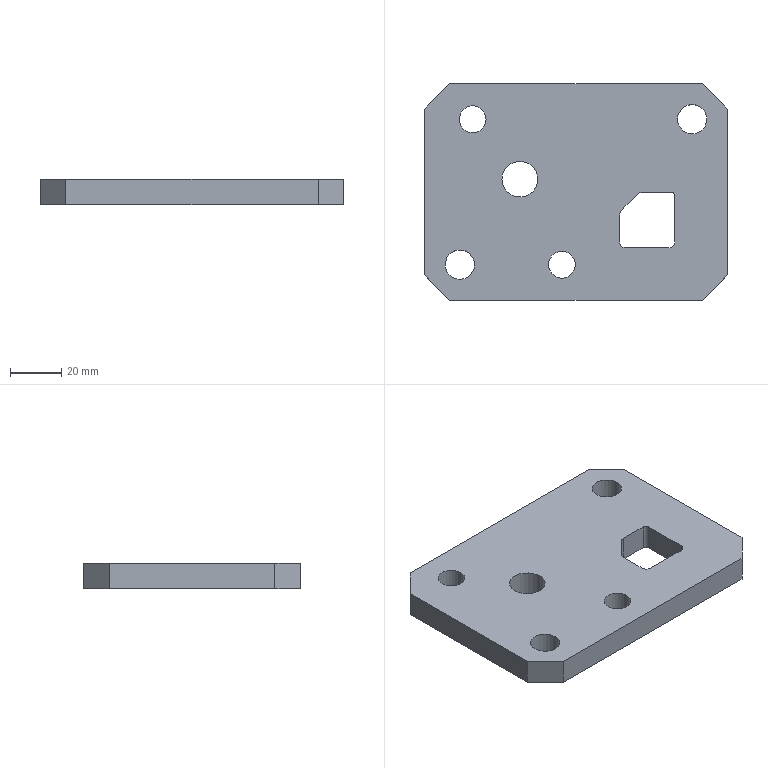Part | NX | features 23 2 | 1 solid | 25 faces | box 119 x 85 x 10 mm | volume 89428 mm3 | plane 15 | cylinder 10 | commonest cylinder face diameters 4.6 x2 5.6 x2 10.5 x2 11.509 x2 3 x1 14 x1
STEP:
#1=CARTESIAN_POINT('',(80.029,-411.95,-33.5));
#2=VERTEX_POINT('',#1);
#3=CARTESIAN_POINT('',(87.029,-411.95,-33.5));
#4=DIRECTION('',(0.,0.,-1.));
#5=DIRECTION('',(-1.,0.,0.));
#6=AXIS2_PLACEMENT_3D('',#3,#4,#5);
#7=CIRCLE('',#6,7.);
#8=EDGE_CURVE('',#2,#2,#7,.T.);
#9=ORIENTED_EDGE('',*,*,#8,.F.);
#10=EDGE_LOOP('',(#9));
#11=FACE_BOUND('',#10,.T.);
#12=CARTESIAN_POINT('',(80.029,-411.95,-43.5));
#13=VERTEX_POINT('',#12);
#14=CARTESIAN_POINT('',(87.029,-411.95,-43.5));
#15=DIRECTION('',(0.,0.,-1.));
#16=DIRECTION('',(-1.,0.,0.));
#17=AXIS2_PLACEMENT_3D('',#14,#15,#16);
#18=CIRCLE('',#17,7.);
#19=EDGE_CURVE('',#13,#13,#18,.T.);
#20=ORIENTED_EDGE('',*,*,#19,.T.);
#21=EDGE_LOOP('',(#20));
#22=FACE_BOUND('',#21,.T.);
#23=CARTESIAN_POINT('',(87.029,-411.95,-33.5));
#24=DIRECTION('',(0.,0.,1.));
#25=DIRECTION('',(1.,0.,0.));
#26=AXIS2_PLACEMENT_3D('',#23,#24,#25);
#27=CYLINDRICAL_SURFACE('',#26,7.);
#28=ADVANCED_FACE('',(#11,#22),#27,.F.);
#29=CARTESIAN_POINT('',(49.529,-449.45,-33.5));
#30=VERTEX_POINT('',#29);
#31=CARTESIAN_POINT('',(49.529,-384.45,-33.5));
#32=VERTEX_POINT('',#31);
#33=CARTESIAN_POINT('',(49.529,-411.95,-33.5));
#34=DIRECTION('',(0.,1.,0.));
#35=VECTOR('',#34,1000.);
#36=LINE('',#33,#35);
#37=EDGE_CURVE('',#30,#32,#36,.T.);
#38=ORIENTED_EDGE('',*,*,#37,.T.);
#39=CARTESIAN_POINT('',(49.529,-384.45,-43.5));
#40=VERTEX_POINT('',#39);
#41=CARTESIAN_POINT('',(49.529,-384.45,-33.5));
#42=DIRECTION('',(0.,0.,1.));
#43=VECTOR('',#42,1000.);
#44=LINE('',#41,#43);
#45=EDGE_CURVE('',#40,#32,#44,.T.);
#46=ORIENTED_EDGE('',*,*,#45,.F.);
#47=CARTESIAN_POINT('',(49.529,-449.45,-43.5));
#48=VERTEX_POINT('',#47);
#49=CARTESIAN_POINT('',(49.529,-377.506,-43.5));
#50=DIRECTION('',(0.,1.,0.));
#51=VECTOR('',#50,1000.);
#52=LINE('',#49,#51);
#53=EDGE_CURVE('',#48,#40,#52,.T.);
#54=ORIENTED_EDGE('',*,*,#53,.F.);
#55=CARTESIAN_POINT('',(49.529,-449.45,-33.5));
#56=DIRECTION('',(0.,0.,-1.));
#57=VECTOR('',#56,1000.);
#58=LINE('',#55,#57);
#59=EDGE_CURVE('',#30,#48,#58,.T.);
#60=ORIENTED_EDGE('',*,*,#59,.F.);
#61=EDGE_LOOP('',(#38,#46,#54,#60));
#62=FACE_BOUND('',#61,.T.);
#63=CARTESIAN_POINT('',(49.529,-411.95,-33.5));
#64=DIRECTION('',(1.,0.,0.));
#65=DIRECTION('',(0.,1.,0.));
#66=AXIS2_PLACEMENT_3D('',#63,#64,#65);
#67=PLANE('',#66);
#68=ADVANCED_FACE('',(#62),#67,.F.);
#69=CARTESIAN_POINT('',(158.529,-459.45,-33.5));
#70=VERTEX_POINT('',#69);
#71=CARTESIAN_POINT('',(59.529,-459.45,-33.5));
#72=VERTEX_POINT('',#71);
#73=CARTESIAN_POINT('',(87.029,-459.45,-33.5));
#74=DIRECTION('',(-1.,0.,0.));
#75=VECTOR('',#74,1000.);
#76=LINE('',#73,#75);
#77=EDGE_CURVE('',#70,#72,#76,.T.);
#78=ORIENTED_EDGE('',*,*,#77,.T.);
#79=CARTESIAN_POINT('',(59.529,-459.45,-43.5));
#80=VERTEX_POINT('',#79);
#81=CARTESIAN_POINT('',(59.529,-459.45,-33.5));
#82=DIRECTION('',(0.,0.,1.));
#83=VECTOR('',#82,1000.);
#84=LINE('',#81,#83);
#85=EDGE_CURVE('',#80,#72,#84,.T.);
#86=ORIENTED_EDGE('',*,*,#85,.F.);
#87=CARTESIAN_POINT('',(158.529,-459.45,-43.5));
#88=VERTEX_POINT('',#87);
#89=CARTESIAN_POINT('',(119.455,-459.45,-43.5));
#90=DIRECTION('',(-1.,0.,0.));
#91=VECTOR('',#90,1000.);
#92=LINE('',#89,#91);
#93=EDGE_CURVE('',#88,#80,#92,.T.);
#94=ORIENTED_EDGE('',*,*,#93,.F.);
#95=CARTESIAN_POINT('',(158.529,-459.45,-33.5));
#96=DIRECTION('',(0.,0.,-1.));
#97=VECTOR('',#96,1000.);
#98=LINE('',#95,#97);
#99=EDGE_CURVE('',#70,#88,#98,.T.);
#100=ORIENTED_EDGE('',*,*,#99,.F.);
#101=EDGE_LOOP('',(#78,#86,#94,#100));
#102=FACE_BOUND('',#101,.T.);
#103=CARTESIAN_POINT('',(87.029,-459.45,-33.5));
#104=DIRECTION('',(0.,1.,0.));
#105=DIRECTION('',(-1.,0.,0.));
#106=AXIS2_PLACEMENT_3D('',#103,#104,#105);
#107=PLANE('',#106);
#108=ADVANCED_FACE('',(#102),#107,.F.);
#109=CARTESIAN_POINT('',(168.529,-384.45,-33.5));
#110=VERTEX_POINT('',#109);
#111=CARTESIAN_POINT('',(168.529,-449.45,-33.5));
#112=VERTEX_POINT('',#111);
#113=CARTESIAN_POINT('',(168.529,-411.95,-33.5));
#114=DIRECTION('',(0.,-1.,0.));
#115=VECTOR('',#114,1000.);
#116=LINE('',#113,#115);
#117=EDGE_CURVE('',#110,#112,#116,.T.);
#118=ORIENTED_EDGE('',*,*,#117,.T.);
#119=CARTESIAN_POINT('',(168.529,-449.45,-43.5));
#120=VERTEX_POINT('',#119);
#121=CARTESIAN_POINT('',(168.529,-449.45,-33.5));
#122=DIRECTION('',(0.,0.,1.));
#123=VECTOR('',#122,1000.);
#124=LINE('',#121,#123);
#125=EDGE_CURVE('',#120,#112,#124,.T.);
#126=ORIENTED_EDGE('',*,*,#125,.F.);
#127=CARTESIAN_POINT('',(168.529,-384.45,-43.5));
#128=VERTEX_POINT('',#127);
#129=CARTESIAN_POINT('',(168.529,-377.506,-43.5));
#130=DIRECTION('',(0.,-1.,0.));
#131=VECTOR('',#130,1000.);
#132=LINE('',#129,#131);
#133=EDGE_CURVE('',#128,#120,#132,.T.);
#134=ORIENTED_EDGE('',*,*,#133,.F.);
#135=CARTESIAN_POINT('',(168.529,-384.45,-33.5));
#136=DIRECTION('',(0.,0.,-1.));
#137=VECTOR('',#136,1000.);
#138=LINE('',#135,#137);
#139=EDGE_CURVE('',#110,#128,#138,.T.);
#140=ORIENTED_EDGE('',*,*,#139,.F.);
#141=EDGE_LOOP('',(#118,#126,#134,#140));
#142=FACE_BOUND('',#141,.T.);
#143=CARTESIAN_POINT('',(168.529,-411.95,-33.5));
#144=DIRECTION('',(-1.,0.,0.));
#145=DIRECTION('',(0.,-1.,0.));
#146=AXIS2_PLACEMENT_3D('',#143,#144,#145);
#147=PLANE('',#146);
#148=ADVANCED_FACE('',(#142),#147,.F.);
#149=CARTESIAN_POINT('',(63.279,-388.45,-43.5));
#150=VERTEX_POINT('',#149);
#151=CARTESIAN_POINT('',(68.529,-388.45,-43.5));
#152=DIRECTION('',(0.,0.,1.));
#153=DIRECTION('',(-1.,0.,0.));
#154=AXIS2_PLACEMENT_3D('',#151,#152,#153);
#155=CIRCLE('',#154,5.25);
#156=EDGE_CURVE('',#150,#150,#155,.T.);
#157=ORIENTED_EDGE('',*,*,#156,.F.);
#158=EDGE_LOOP('',(#157));
#159=FACE_BOUND('',#158,.T.);
#160=CARTESIAN_POINT('',(63.279,-388.45,-33.5));
#161=VERTEX_POINT('',#160);
#162=CARTESIAN_POINT('',(68.529,-388.45,-33.5));
#163=DIRECTION('',(0.,0.,1.));
#164=DIRECTION('',(-1.,0.,0.));
#165=AXIS2_PLACEMENT_3D('',#162,#163,#164);
#166=CIRCLE('',#165,5.25);
#167=EDGE_CURVE('',#161,#161,#166,.T.);
#168=ORIENTED_EDGE('',*,*,#167,.T.);
#169=EDGE_LOOP('',(#168));
#170=FACE_BOUND('',#169,.T.);
#171=CARTESIAN_POINT('',(68.529,-388.45,-33.5));
#172=DIRECTION('',(0.,0.,-1.));
#173=DIRECTION('',(-1.,0.,0.));
#174=AXIS2_PLACEMENT_3D('',#171,#172,#173);
#175=CYLINDRICAL_SURFACE('',#174,5.25);
#176=ADVANCED_FACE('',(#159,#170),#175,.F.);
#177=CARTESIAN_POINT('',(57.774,-445.45,-43.5));
#178=VERTEX_POINT('',#177);
#179=CARTESIAN_POINT('',(63.529,-445.45,-43.5));
#180=DIRECTION('',(0.,0.,1.));
#181=DIRECTION('',(-1.,0.,0.));
#182=AXIS2_PLACEMENT_3D('',#179,#180,#181);
#183=CIRCLE('',#182,5.755);
#184=EDGE_CURVE('',#178,#178,#183,.T.);
#185=ORIENTED_EDGE('',*,*,#184,.F.);
#186=EDGE_LOOP('',(#185));
#187=FACE_BOUND('',#186,.T.);
#188=CARTESIAN_POINT('',(57.774,-445.45,-33.5));
#189=VERTEX_POINT('',#188);
#190=CARTESIAN_POINT('',(63.529,-445.45,-33.5));
#191=DIRECTION('',(0.,0.,1.));
#192=DIRECTION('',(-1.,0.,0.));
#193=AXIS2_PLACEMENT_3D('',#190,#191,#192);
#194=CIRCLE('',#193,5.755);
#195=EDGE_CURVE('',#189,#189,#194,.T.);
#196=ORIENTED_EDGE('',*,*,#195,.T.);
#197=EDGE_LOOP('',(#196));
#198=FACE_BOUND('',#197,.T.);
#199=CARTESIAN_POINT('',(63.529,-445.45,-33.5));
#200=DIRECTION('',(0.,0.,-1.));
#201=DIRECTION('',(-1.,0.,0.));
#202=AXIS2_PLACEMENT_3D('',#199,#200,#201);
#203=CYLINDRICAL_SURFACE('',#202,5.755);
#204=ADVANCED_FACE('',(#187,#198),#203,.F.);
#205=CARTESIAN_POINT('',(98.279,-445.45,-43.5));
#206=VERTEX_POINT('',#205);
#207=CARTESIAN_POINT('',(103.529,-445.45,-43.5));
#208=DIRECTION('',(0.,0.,1.));
#209=DIRECTION('',(-1.,0.,0.));
#210=AXIS2_PLACEMENT_3D('',#207,#208,#209);
#211=CIRCLE('',#210,5.25);
#212=EDGE_CURVE('',#206,#206,#211,.T.);
#213=ORIENTED_EDGE('',*,*,#212,.F.);
#214=EDGE_LOOP('',(#213));
#215=FACE_BOUND('',#214,.T.);
#216=CARTESIAN_POINT('',(98.279,-445.45,-33.5));
#217=VERTEX_POINT('',#216);
#218=CARTESIAN_POINT('',(103.529,-445.45,-33.5));
#219=DIRECTION('',(0.,0.,1.));
#220=DIRECTION('',(-1.,0.,0.));
#221=AXIS2_PLACEMENT_3D('',#218,#219,#220);
#222=CIRCLE('',#221,5.25);
#223=EDGE_CURVE('',#217,#217,#222,.T.);
#224=ORIENTED_EDGE('',*,*,#223,.T.);
#225=EDGE_LOOP('',(#224));
#226=FACE_BOUND('',#225,.T.);
#227=CARTESIAN_POINT('',(103.529,-445.45,-33.5));
#228=DIRECTION('',(0.,0.,-1.));
#229=DIRECTION('',(-1.,0.,0.));
#230=AXIS2_PLACEMENT_3D('',#227,#228,#229);
#231=CYLINDRICAL_SURFACE('',#230,5.25);
#232=ADVANCED_FACE('',(#215,#226),#231,.F.);
#233=CARTESIAN_POINT('',(148.774,-388.45,-43.5));
#234=VERTEX_POINT('',#233);
#235=CARTESIAN_POINT('',(154.529,-388.45,-43.5));
#236=DIRECTION('',(0.,0.,1.));
#237=DIRECTION('',(-1.,0.,0.));
#238=AXIS2_PLACEMENT_3D('',#235,#236,#237);
#239=CIRCLE('',#238,5.755);
#240=EDGE_CURVE('',#234,#234,#239,.T.);
#241=ORIENTED_EDGE('',*,*,#240,.F.);
#242=EDGE_LOOP('',(#241));
#243=FACE_BOUND('',#242,.T.);
#244=CARTESIAN_POINT('',(148.774,-388.45,-33.5));
#245=VERTEX_POINT('',#244);
#246=CARTESIAN_POINT('',(154.529,-388.45,-33.5));
#247=DIRECTION('',(0.,0.,1.));
#248=DIRECTION('',(-1.,0.,0.));
#249=AXIS2_PLACEMENT_3D('',#246,#247,#248);
#250=CIRCLE('',#249,5.755);
#251=EDGE_CURVE('',#245,#245,#250,.T.);
#252=ORIENTED_EDGE('',*,*,#251,.T.);
#253=EDGE_LOOP('',(#252));
#254=FACE_BOUND('',#253,.T.);
#255=CARTESIAN_POINT('',(154.529,-388.45,-33.5));
#256=DIRECTION('',(0.,0.,-1.));
#257=DIRECTION('',(-1.,0.,0.));
#258=AXIS2_PLACEMENT_3D('',#255,#256,#257);
#259=CYLINDRICAL_SURFACE('',#258,5.755);
#260=ADVANCED_FACE('',(#243,#254),#259,.F.);
#261=CARTESIAN_POINT('',(59.529,-374.45,-43.5));
#262=VERTEX_POINT('',#261);
#263=CARTESIAN_POINT('',(158.529,-374.45,-43.5));
#264=VERTEX_POINT('',#263);
#265=CARTESIAN_POINT('',(119.455,-374.45,-43.5));
#266=DIRECTION('',(1.,0.,0.));
#267=VECTOR('',#266,1000.);
#268=LINE('',#265,#267);
#269=EDGE_CURVE('',#262,#264,#268,.T.);
#270=ORIENTED_EDGE('',*,*,#269,.F.);
#271=CARTESIAN_POINT('',(59.529,-374.45,-33.5));
#272=VERTEX_POINT('',#271);
#273=CARTESIAN_POINT('',(59.529,-374.45,-33.5));
#274=DIRECTION('',(0.,0.,-1.));
#275=VECTOR('',#274,1000.);
#276=LINE('',#273,#275);
#277=EDGE_CURVE('',#272,#262,#276,.T.);
#278=ORIENTED_EDGE('',*,*,#277,.F.);
#279=CARTESIAN_POINT('',(158.529,-374.45,-33.5));
#280=VERTEX_POINT('',#279);
#281=CARTESIAN_POINT('',(87.029,-374.45,-33.5));
#282=DIRECTION('',(1.,0.,0.));
#283=VECTOR('',#282,1000.);
#284=LINE('',#281,#283);
#285=EDGE_CURVE('',#272,#280,#284,.T.);
#286=ORIENTED_EDGE('',*,*,#285,.T.);
#287=CARTESIAN_POINT('',(158.529,-374.45,-33.5));
#288=DIRECTION('',(0.,0.,1.));
#289=VECTOR('',#288,1000.);
#290=LINE('',#287,#289);
#291=EDGE_CURVE('',#264,#280,#290,.T.);
#292=ORIENTED_EDGE('',*,*,#291,.F.);
#293=EDGE_LOOP('',(#270,#278,#286,#292));
#294=FACE_BOUND('',#293,.T.);
#295=CARTESIAN_POINT('',(87.029,-374.45,-33.5));
#296=DIRECTION('',(0.,-1.,0.));
#297=DIRECTION('',(1.,0.,0.));
#298=AXIS2_PLACEMENT_3D('',#295,#296,#297);
#299=PLANE('',#298);
#300=ADVANCED_FACE('',(#294),#299,.F.);
#301=CARTESIAN_POINT('',(133.172,-417.82,-43.5));
#302=VERTEX_POINT('',#301);
#303=CARTESIAN_POINT('',(135.152,-417.,-43.5));
#304=VERTEX_POINT('',#303);
#305=CARTESIAN_POINT('',(135.152,-419.8,-43.5));
#306=DIRECTION('',(0.,0.,-1.));
#307=DIRECTION('',(-1.,0.,0.));
#308=AXIS2_PLACEMENT_3D('',#305,#306,#307);
#309=CIRCLE('',#308,2.8);
#310=EDGE_CURVE('',#302,#304,#309,.T.);
#311=ORIENTED_EDGE('',*,*,#310,.F.);
#312=CARTESIAN_POINT('',(126.942,-424.05,-43.5));
#313=VERTEX_POINT('',#312);
#314=CARTESIAN_POINT('',(146.47,-404.522,-43.5));
#315=DIRECTION('',(-0.7071,-0.7071,0.));
#316=VECTOR('',#315,1000.);
#317=LINE('',#314,#316);
#318=EDGE_CURVE('',#302,#313,#317,.T.);
#319=ORIENTED_EDGE('',*,*,#318,.T.);
#320=CARTESIAN_POINT('',(126.122,-426.03,-43.5));
#321=VERTEX_POINT('',#320);
#322=CARTESIAN_POINT('',(128.922,-426.03,-43.5));
#323=DIRECTION('',(0.,0.,-1.));
#324=DIRECTION('',(-1.,0.,0.));
#325=AXIS2_PLACEMENT_3D('',#322,#323,#324);
#326=CIRCLE('',#325,2.8);
#327=EDGE_CURVE('',#321,#313,#326,.T.);
#328=ORIENTED_EDGE('',*,*,#327,.F.);
#329=CARTESIAN_POINT('',(126.122,-436.51,-43.5));
#330=VERTEX_POINT('',#329);
#331=CARTESIAN_POINT('',(126.122,-377.506,-43.5));
#332=DIRECTION('',(0.,-1.,0.));
#333=VECTOR('',#332,1000.);
#334=LINE('',#331,#333);
#335=EDGE_CURVE('',#321,#330,#334,.T.);
#336=ORIENTED_EDGE('',*,*,#335,.T.);
#337=CARTESIAN_POINT('',(128.422,-438.81,-43.5));
#338=VERTEX_POINT('',#337);
#339=CARTESIAN_POINT('',(128.422,-436.51,-43.5));
#340=DIRECTION('',(0.,0.,-1.));
#341=DIRECTION('',(-1.,0.,0.));
#342=AXIS2_PLACEMENT_3D('',#339,#340,#341);
#343=CIRCLE('',#342,2.3);
#344=EDGE_CURVE('',#338,#330,#343,.T.);
#345=ORIENTED_EDGE('',*,*,#344,.F.);
#346=CARTESIAN_POINT('',(145.422,-438.81,-43.5));
#347=VERTEX_POINT('',#346);
#348=CARTESIAN_POINT('',(119.455,-438.81,-43.5));
#349=DIRECTION('',(1.,0.,0.));
#350=VECTOR('',#349,1000.);
#351=LINE('',#348,#350);
#352=EDGE_CURVE('',#338,#347,#351,.T.);
#353=ORIENTED_EDGE('',*,*,#352,.T.);
#354=CARTESIAN_POINT('',(147.722,-436.51,-43.5));
#355=VERTEX_POINT('',#354);
#356=CARTESIAN_POINT('',(145.422,-436.51,-43.5));
#357=DIRECTION('',(0.,0.,-1.));
#358=DIRECTION('',(-1.,0.,0.));
#359=AXIS2_PLACEMENT_3D('',#356,#357,#358);
#360=CIRCLE('',#359,2.3);
#361=EDGE_CURVE('',#355,#347,#360,.T.);
#362=ORIENTED_EDGE('',*,*,#361,.F.);
#363=CARTESIAN_POINT('',(147.722,-418.5,-43.5));
#364=VERTEX_POINT('',#363);
#365=CARTESIAN_POINT('',(147.722,-377.506,-43.5));
#366=DIRECTION('',(0.,1.,0.));
#367=VECTOR('',#366,1000.);
#368=LINE('',#365,#367);
#369=EDGE_CURVE('',#355,#364,#368,.T.);
#370=ORIENTED_EDGE('',*,*,#369,.T.);
#371=CARTESIAN_POINT('',(146.222,-417.,-43.5));
#372=VERTEX_POINT('',#371);
#373=CARTESIAN_POINT('',(146.222,-418.5,-43.5));
#374=DIRECTION('',(0.,0.,-1.));
#375=DIRECTION('',(-1.,0.,0.));
#376=AXIS2_PLACEMENT_3D('',#373,#374,#375);
#377=CIRCLE('',#376,1.5);
#378=EDGE_CURVE('',#372,#364,#377,.T.);
#379=ORIENTED_EDGE('',*,*,#378,.F.);
#380=CARTESIAN_POINT('',(119.455,-417.,-43.5));
#381=DIRECTION('',(1.,0.,0.));
#382=VECTOR('',#381,1000.);
#383=LINE('',#380,#382);
#384=EDGE_CURVE('',#304,#372,#383,.T.);
#385=ORIENTED_EDGE('',*,*,#384,.F.);
#386=EDGE_LOOP('',(#311,#319,#328,#336,#345,#353,#362,#370,#379,#385));
#387=FACE_BOUND('',#386,.T.);
#388=ORIENTED_EDGE('',*,*,#156,.T.);
#389=EDGE_LOOP('',(#388));
#390=FACE_BOUND('',#389,.T.);
#391=ORIENTED_EDGE('',*,*,#184,.T.);
#392=EDGE_LOOP('',(#391));
#393=FACE_BOUND('',#392,.T.);
#394=ORIENTED_EDGE('',*,*,#212,.T.);
#395=EDGE_LOOP('',(#394));
#396=FACE_BOUND('',#395,.T.);
#397=ORIENTED_EDGE('',*,*,#240,.T.);
#398=EDGE_LOOP('',(#397));
#399=FACE_BOUND('',#398,.T.);
#400=ORIENTED_EDGE('',*,*,#133,.T.);
#401=CARTESIAN_POINT('',(199.464,-418.515,-43.5));
#402=DIRECTION('',(0.7071,0.7071,0.));
#403=VECTOR('',#402,1000.);
#404=LINE('',#401,#403);
#405=EDGE_CURVE('',#88,#120,#404,.T.);
#406=ORIENTED_EDGE('',*,*,#405,.F.);
#407=ORIENTED_EDGE('',*,*,#93,.T.);
#408=CARTESIAN_POINT('',(51.02,-450.941,-43.5));
#409=DIRECTION('',(0.7071,-0.7071,0.));
#410=VECTOR('',#409,1000.);
#411=LINE('',#408,#410);
#412=EDGE_CURVE('',#48,#80,#411,.T.);
#413=ORIENTED_EDGE('',*,*,#412,.F.);
#414=ORIENTED_EDGE('',*,*,#53,.T.);
#415=CARTESIAN_POINT('',(85.464,-348.515,-43.5));
#416=DIRECTION('',(-0.7071,-0.7071,0.));
#417=VECTOR('',#416,1000.);
#418=LINE('',#415,#417);
#419=EDGE_CURVE('',#262,#40,#418,.T.);
#420=ORIENTED_EDGE('',*,*,#419,.F.);
#421=ORIENTED_EDGE('',*,*,#269,.T.);
#422=CARTESIAN_POINT('',(165.02,-380.941,-43.5));
#423=DIRECTION('',(-0.7071,0.7071,0.));
#424=VECTOR('',#423,1000.);
#425=LINE('',#422,#424);
#426=EDGE_CURVE('',#128,#264,#425,.T.);
#427=ORIENTED_EDGE('',*,*,#426,.F.);
#428=EDGE_LOOP('',(#400,#406,#407,#413,#414,#420,#421,#427));
#429=FACE_BOUND('',#428,.T.);
#430=ORIENTED_EDGE('',*,*,#19,.F.);
#431=EDGE_LOOP('',(#430));
#432=FACE_BOUND('',#431,.T.);
#433=CARTESIAN_POINT('',(119.455,-377.506,-43.5));
#434=DIRECTION('',(0.,0.,-1.));
#435=DIRECTION('',(-1.,0.,0.));
#436=AXIS2_PLACEMENT_3D('',#433,#434,#435);
#437=PLANE('',#436);
#438=ADVANCED_FACE('',(#387,#390,#393,#396,#399,#429,#432),#437,.T.);
#439=CARTESIAN_POINT('',(133.172,-417.82,-33.5));
#440=VERTEX_POINT('',#439);
#441=CARTESIAN_POINT('',(126.942,-424.05,-33.5));
#442=VERTEX_POINT('',#441);
#443=CARTESIAN_POINT('',(146.47,-404.522,-33.5));
#444=DIRECTION('',(-0.7071,-0.7071,0.));
#445=VECTOR('',#444,1000.);
#446=LINE('',#443,#445);
#447=EDGE_CURVE('',#440,#442,#446,.T.);
#448=ORIENTED_EDGE('',*,*,#447,.F.);
#449=CARTESIAN_POINT('',(135.152,-417.,-33.5));
#450=VERTEX_POINT('',#449);
#451=CARTESIAN_POINT('',(135.152,-419.8,-33.5));
#452=DIRECTION('',(0.,0.,-1.));
#453=DIRECTION('',(-1.,0.,0.));
#454=AXIS2_PLACEMENT_3D('',#451,#452,#453);
#455=CIRCLE('',#454,2.8);
#456=EDGE_CURVE('',#440,#450,#455,.T.);
#457=ORIENTED_EDGE('',*,*,#456,.T.);
#458=CARTESIAN_POINT('',(146.222,-417.,-33.5));
#459=VERTEX_POINT('',#458);
#460=CARTESIAN_POINT('',(119.455,-417.,-33.5));
#461=DIRECTION('',(1.,0.,0.));
#462=VECTOR('',#461,1000.);
#463=LINE('',#460,#462);
#464=EDGE_CURVE('',#450,#459,#463,.T.);
#465=ORIENTED_EDGE('',*,*,#464,.T.);
#466=CARTESIAN_POINT('',(147.722,-418.5,-33.5));
#467=VERTEX_POINT('',#466);
#468=CARTESIAN_POINT('',(146.222,-418.5,-33.5));
#469=DIRECTION('',(0.,0.,-1.));
#470=DIRECTION('',(-1.,0.,0.));
#471=AXIS2_PLACEMENT_3D('',#468,#469,#470);
#472=CIRCLE('',#471,1.5);
#473=EDGE_CURVE('',#459,#467,#472,.T.);
#474=ORIENTED_EDGE('',*,*,#473,.T.);
#475=CARTESIAN_POINT('',(147.722,-436.51,-33.5));
#476=VERTEX_POINT('',#475);
#477=CARTESIAN_POINT('',(147.722,-377.506,-33.5));
#478=DIRECTION('',(0.,1.,0.));
#479=VECTOR('',#478,1000.);
#480=LINE('',#477,#479);
#481=EDGE_CURVE('',#476,#467,#480,.T.);
#482=ORIENTED_EDGE('',*,*,#481,.F.);
#483=CARTESIAN_POINT('',(145.422,-438.81,-33.5));
#484=VERTEX_POINT('',#483);
#485=CARTESIAN_POINT('',(145.422,-436.51,-33.5));
#486=DIRECTION('',(0.,0.,-1.));
#487=DIRECTION('',(-1.,0.,0.));
#488=AXIS2_PLACEMENT_3D('',#485,#486,#487);
#489=CIRCLE('',#488,2.3);
#490=EDGE_CURVE('',#476,#484,#489,.T.);
#491=ORIENTED_EDGE('',*,*,#490,.T.);
#492=CARTESIAN_POINT('',(128.422,-438.81,-33.5));
#493=VERTEX_POINT('',#492);
#494=CARTESIAN_POINT('',(119.455,-438.81,-33.5));
#495=DIRECTION('',(1.,0.,0.));
#496=VECTOR('',#495,1000.);
#497=LINE('',#494,#496);
#498=EDGE_CURVE('',#493,#484,#497,.T.);
#499=ORIENTED_EDGE('',*,*,#498,.F.);
#500=CARTESIAN_POINT('',(126.122,-436.51,-33.5));
#501=VERTEX_POINT('',#500);
#502=CARTESIAN_POINT('',(128.422,-436.51,-33.5));
#503=DIRECTION('',(0.,0.,-1.));
#504=DIRECTION('',(-1.,0.,0.));
#505=AXIS2_PLACEMENT_3D('',#502,#503,#504);
#506=CIRCLE('',#505,2.3);
#507=EDGE_CURVE('',#493,#501,#506,.T.);
#508=ORIENTED_EDGE('',*,*,#507,.T.);
#509=CARTESIAN_POINT('',(126.122,-426.03,-33.5));
#510=VERTEX_POINT('',#509);
#511=CARTESIAN_POINT('',(126.122,-377.506,-33.5));
#512=DIRECTION('',(0.,-1.,0.));
#513=VECTOR('',#512,1000.);
#514=LINE('',#511,#513);
#515=EDGE_CURVE('',#510,#501,#514,.T.);
#516=ORIENTED_EDGE('',*,*,#515,.F.);
#517=CARTESIAN_POINT('',(128.922,-426.03,-33.5));
#518=DIRECTION('',(0.,0.,-1.));
#519=DIRECTION('',(-1.,0.,0.));
#520=AXIS2_PLACEMENT_3D('',#517,#518,#519);
#521=CIRCLE('',#520,2.8);
#522=EDGE_CURVE('',#510,#442,#521,.T.);
#523=ORIENTED_EDGE('',*,*,#522,.T.);
#524=EDGE_LOOP('',(#448,#457,#465,#474,#482,#491,#499,#508,#516,#523));
#525=FACE_BOUND('',#524,.T.);
#526=ORIENTED_EDGE('',*,*,#167,.F.);
#527=EDGE_LOOP('',(#526));
#528=FACE_BOUND('',#527,.T.);
#529=ORIENTED_EDGE('',*,*,#195,.F.);
#530=EDGE_LOOP('',(#529));
#531=FACE_BOUND('',#530,.T.);
#532=ORIENTED_EDGE('',*,*,#223,.F.);
#533=EDGE_LOOP('',(#532));
#534=FACE_BOUND('',#533,.T.);
#535=ORIENTED_EDGE('',*,*,#251,.F.);
#536=EDGE_LOOP('',(#535));
#537=FACE_BOUND('',#536,.T.);
#538=ORIENTED_EDGE('',*,*,#285,.F.);
#539=CARTESIAN_POINT('',(54.529,-379.45,-33.5));
#540=DIRECTION('',(0.7071,0.7071,0.));
#541=VECTOR('',#540,1000.);
#542=LINE('',#539,#541);
#543=EDGE_CURVE('',#32,#272,#542,.T.);
#544=ORIENTED_EDGE('',*,*,#543,.F.);
#545=ORIENTED_EDGE('',*,*,#37,.F.);
#546=CARTESIAN_POINT('',(49.529,-449.45,-33.5));
#547=DIRECTION('',(-0.7071,0.7071,0.));
#548=VECTOR('',#547,1000.);
#549=LINE('',#546,#548);
#550=EDGE_CURVE('',#72,#30,#549,.T.);
#551=ORIENTED_EDGE('',*,*,#550,.F.);
#552=ORIENTED_EDGE('',*,*,#77,.F.);
#553=CARTESIAN_POINT('',(163.529,-454.45,-33.5));
#554=DIRECTION('',(-0.7071,-0.7071,0.));
#555=VECTOR('',#554,1000.);
#556=LINE('',#553,#555);
#557=EDGE_CURVE('',#112,#70,#556,.T.);
#558=ORIENTED_EDGE('',*,*,#557,.F.);
#559=ORIENTED_EDGE('',*,*,#117,.F.);
#560=CARTESIAN_POINT('',(168.529,-384.45,-33.5));
#561=DIRECTION('',(0.7071,-0.7071,0.));
#562=VECTOR('',#561,1000.);
#563=LINE('',#560,#562);
#564=EDGE_CURVE('',#280,#110,#563,.T.);
#565=ORIENTED_EDGE('',*,*,#564,.F.);
#566=EDGE_LOOP('',(#538,#544,#545,#551,#552,#558,#559,#565));
#567=FACE_BOUND('',#566,.T.);
#568=ORIENTED_EDGE('',*,*,#8,.T.);
#569=EDGE_LOOP('',(#568));
#570=FACE_BOUND('',#569,.T.);
#571=CARTESIAN_POINT('',(119.455,-377.506,-33.5));
#572=DIRECTION('',(0.,0.,-1.));
#573=DIRECTION('',(-1.,0.,0.));
#574=AXIS2_PLACEMENT_3D('',#571,#572,#573);
#575=PLANE('',#574);
#576=ADVANCED_FACE('',(#525,#528,#531,#534,#537,#567,#570),#575,.F.);
#577=ORIENTED_EDGE('',*,*,#564,.T.);
#578=ORIENTED_EDGE('',*,*,#139,.T.);
#579=ORIENTED_EDGE('',*,*,#426,.T.);
#580=ORIENTED_EDGE('',*,*,#291,.T.);
#581=EDGE_LOOP('',(#577,#578,#579,#580));
#582=FACE_BOUND('',#581,.T.);
#583=CARTESIAN_POINT('',(168.529,-384.45,-33.5));
#584=DIRECTION('',(-0.7071,-0.7071,0.));
#585=DIRECTION('',(0.,0.,-1.));
#586=AXIS2_PLACEMENT_3D('',#583,#584,#585);
#587=PLANE('',#586);
#588=ADVANCED_FACE('',(#582),#587,.F.);
#589=ORIENTED_EDGE('',*,*,#557,.T.);
#590=ORIENTED_EDGE('',*,*,#99,.T.);
#591=ORIENTED_EDGE('',*,*,#405,.T.);
#592=ORIENTED_EDGE('',*,*,#125,.T.);
#593=EDGE_LOOP('',(#589,#590,#591,#592));
#594=FACE_BOUND('',#593,.T.);
#595=CARTESIAN_POINT('',(163.529,-454.45,-33.5));
#596=DIRECTION('',(-0.7071,0.7071,0.));
#597=DIRECTION('',(0.,0.,-1.));
#598=AXIS2_PLACEMENT_3D('',#595,#596,#597);
#599=PLANE('',#598);
#600=ADVANCED_FACE('',(#594),#599,.F.);
#601=ORIENTED_EDGE('',*,*,#550,.T.);
#602=ORIENTED_EDGE('',*,*,#59,.T.);
#603=ORIENTED_EDGE('',*,*,#412,.T.);
#604=ORIENTED_EDGE('',*,*,#85,.T.);
#605=EDGE_LOOP('',(#601,#602,#603,#604));
#606=FACE_BOUND('',#605,.T.);
#607=CARTESIAN_POINT('',(49.529,-449.45,-33.5));
#608=DIRECTION('',(0.7071,0.7071,0.));
#609=DIRECTION('',(0.,0.,-1.));
#610=AXIS2_PLACEMENT_3D('',#607,#608,#609);
#611=PLANE('',#610);
#612=ADVANCED_FACE('',(#606),#611,.F.);
#613=ORIENTED_EDGE('',*,*,#543,.T.);
#614=ORIENTED_EDGE('',*,*,#277,.T.);
#615=ORIENTED_EDGE('',*,*,#419,.T.);
#616=ORIENTED_EDGE('',*,*,#45,.T.);
#617=EDGE_LOOP('',(#613,#614,#615,#616));
#618=FACE_BOUND('',#617,.T.);
#619=CARTESIAN_POINT('',(54.529,-379.45,-33.5));
#620=DIRECTION('',(0.7071,-0.7071,0.));
#621=DIRECTION('',(0.,0.,-1.));
#622=AXIS2_PLACEMENT_3D('',#619,#620,#621);
#623=PLANE('',#622);
#624=ADVANCED_FACE('',(#618),#623,.F.);
#625=ORIENTED_EDGE('',*,*,#384,.T.);
#626=CARTESIAN_POINT('',(146.222,-417.,210.5));
#627=DIRECTION('',(0.,0.,-1.));
#628=VECTOR('',#627,1000.);
#629=LINE('',#626,#628);
#630=EDGE_CURVE('',#459,#372,#629,.T.);
#631=ORIENTED_EDGE('',*,*,#630,.F.);
#632=ORIENTED_EDGE('',*,*,#464,.F.);
#633=CARTESIAN_POINT('',(135.152,-417.,-33.5));
#634=DIRECTION('',(0.,0.,-1.));
#635=VECTOR('',#634,1000.);
#636=LINE('',#633,#635);
#637=EDGE_CURVE('',#450,#304,#636,.T.);
#638=ORIENTED_EDGE('',*,*,#637,.T.);
#639=EDGE_LOOP('',(#625,#631,#632,#638));
#640=FACE_BOUND('',#639,.T.);
#641=CARTESIAN_POINT('',(136.922,-417.,-33.5));
#642=DIRECTION('',(0.,1.,0.));
#643=DIRECTION('',(0.,0.,-1.));
#644=AXIS2_PLACEMENT_3D('',#641,#642,#643);
#645=PLANE('',#644);
#646=ADVANCED_FACE('',(#640),#645,.F.);
#647=CARTESIAN_POINT('',(133.172,-417.82,-48.5));
#648=DIRECTION('',(0.,0.,1.));
#649=VECTOR('',#648,1000.);
#650=LINE('',#647,#649);
#651=EDGE_CURVE('',#302,#440,#650,.T.);
#652=ORIENTED_EDGE('',*,*,#651,.T.);
#653=ORIENTED_EDGE('',*,*,#447,.T.);
#654=CARTESIAN_POINT('',(126.942,-424.05,210.5));
#655=DIRECTION('',(0.,0.,1.));
#656=VECTOR('',#655,1000.);
#657=LINE('',#654,#656);
#658=EDGE_CURVE('',#313,#442,#657,.T.);
#659=ORIENTED_EDGE('',*,*,#658,.F.);
#660=ORIENTED_EDGE('',*,*,#318,.F.);
#661=EDGE_LOOP('',(#652,#653,#659,#660));
#662=FACE_BOUND('',#661,.T.);
#663=CARTESIAN_POINT('',(127.431,-423.561,-48.5));
#664=DIRECTION('',(0.7071,-0.7071,0.));
#665=DIRECTION('',(0.7071,0.7071,0.));
#666=AXIS2_PLACEMENT_3D('',#663,#664,#665);
#667=PLANE('',#666);
#668=ADVANCED_FACE('',(#662),#667,.T.);
#669=ORIENTED_EDGE('',*,*,#310,.T.);
#670=ORIENTED_EDGE('',*,*,#637,.F.);
#671=ORIENTED_EDGE('',*,*,#456,.F.);
#672=ORIENTED_EDGE('',*,*,#651,.F.);
#673=EDGE_LOOP('',(#669,#670,#671,#672));
#674=FACE_BOUND('',#673,.T.);
#675=CARTESIAN_POINT('',(135.152,-419.8,-48.5));
#676=DIRECTION('',(0.,0.,-1.));
#677=DIRECTION('',(1.,0.,0.));
#678=AXIS2_PLACEMENT_3D('',#675,#676,#677);
#679=CYLINDRICAL_SURFACE('',#678,2.8);
#680=ADVANCED_FACE('',(#674),#679,.F.);
#681=ORIENTED_EDGE('',*,*,#327,.T.);
#682=ORIENTED_EDGE('',*,*,#658,.T.);
#683=ORIENTED_EDGE('',*,*,#522,.F.);
#684=CARTESIAN_POINT('',(126.122,-426.03,210.5));
#685=DIRECTION('',(0.,0.,1.));
#686=VECTOR('',#685,1000.);
#687=LINE('',#684,#686);
#688=EDGE_CURVE('',#321,#510,#687,.T.);
#689=ORIENTED_EDGE('',*,*,#688,.F.);
#690=EDGE_LOOP('',(#681,#682,#683,#689));
#691=FACE_BOUND('',#690,.T.);
#692=CARTESIAN_POINT('',(128.922,-426.03,210.5));
#693=DIRECTION('',(0.,0.,-1.));
#694=DIRECTION('',(1.,0.,0.));
#695=AXIS2_PLACEMENT_3D('',#692,#693,#694);
#696=CYLINDRICAL_SURFACE('',#695,2.8);
#697=ADVANCED_FACE('',(#691),#696,.F.);
#698=ORIENTED_EDGE('',*,*,#378,.T.);
#699=CARTESIAN_POINT('',(147.722,-418.5,210.5));
#700=DIRECTION('',(0.,0.,1.));
#701=VECTOR('',#700,1000.);
#702=LINE('',#699,#701);
#703=EDGE_CURVE('',#364,#467,#702,.T.);
#704=ORIENTED_EDGE('',*,*,#703,.T.);
#705=ORIENTED_EDGE('',*,*,#473,.F.);
#706=ORIENTED_EDGE('',*,*,#630,.T.);
#707=EDGE_LOOP('',(#698,#704,#705,#706));
#708=FACE_BOUND('',#707,.T.);
#709=CARTESIAN_POINT('',(146.222,-418.5,210.5));
#710=DIRECTION('',(0.,0.,-1.));
#711=DIRECTION('',(1.,0.,0.));
#712=AXIS2_PLACEMENT_3D('',#709,#710,#711);
#713=CYLINDRICAL_SURFACE('',#712,1.5);
#714=ADVANCED_FACE('',(#708),#713,.F.);
#715=ORIENTED_EDGE('',*,*,#688,.T.);
#716=ORIENTED_EDGE('',*,*,#515,.T.);
#717=CARTESIAN_POINT('',(126.122,-436.51,210.5));
#718=DIRECTION('',(0.,0.,1.));
#719=VECTOR('',#718,1000.);
#720=LINE('',#717,#719);
#721=EDGE_CURVE('',#330,#501,#720,.T.);
#722=ORIENTED_EDGE('',*,*,#721,.F.);
#723=ORIENTED_EDGE('',*,*,#335,.F.);
#724=EDGE_LOOP('',(#715,#716,#722,#723));
#725=FACE_BOUND('',#724,.T.);
#726=CARTESIAN_POINT('',(126.122,-384.125,210.5));
#727=DIRECTION('',(1.,0.,0.));
#728=DIRECTION('',(0.,0.,-1.));
#729=AXIS2_PLACEMENT_3D('',#726,#727,#728);
#730=PLANE('',#729);
#731=ADVANCED_FACE('',(#725),#730,.T.);
#732=CARTESIAN_POINT('',(147.722,-436.51,210.5));
#733=DIRECTION('',(0.,0.,1.));
#734=VECTOR('',#733,1000.);
#735=LINE('',#732,#734);
#736=EDGE_CURVE('',#355,#476,#735,.T.);
#737=ORIENTED_EDGE('',*,*,#736,.T.);
#738=ORIENTED_EDGE('',*,*,#481,.T.);
#739=ORIENTED_EDGE('',*,*,#703,.F.);
#740=ORIENTED_EDGE('',*,*,#369,.F.);
#741=EDGE_LOOP('',(#737,#738,#739,#740));
#742=FACE_BOUND('',#741,.T.);
#743=CARTESIAN_POINT('',(147.722,-384.125,210.5));
#744=DIRECTION('',(-1.,0.,0.));
#745=DIRECTION('',(0.,0.,1.));
#746=AXIS2_PLACEMENT_3D('',#743,#744,#745);
#747=PLANE('',#746);
#748=ADVANCED_FACE('',(#742),#747,.T.);
#749=ORIENTED_EDGE('',*,*,#361,.T.);
#750=CARTESIAN_POINT('',(145.422,-438.81,210.5));
#751=DIRECTION('',(0.,0.,1.));
#752=VECTOR('',#751,1000.);
#753=LINE('',#750,#752);
#754=EDGE_CURVE('',#347,#484,#753,.T.);
#755=ORIENTED_EDGE('',*,*,#754,.T.);
#756=ORIENTED_EDGE('',*,*,#490,.F.);
#757=ORIENTED_EDGE('',*,*,#736,.F.);
#758=EDGE_LOOP('',(#749,#755,#756,#757));
#759=FACE_BOUND('',#758,.T.);
#760=CARTESIAN_POINT('',(145.422,-436.51,210.5));
#761=DIRECTION('',(0.,0.,-1.));
#762=DIRECTION('',(-1.,0.,0.));
#763=AXIS2_PLACEMENT_3D('',#760,#761,#762);
#764=CYLINDRICAL_SURFACE('',#763,2.3);
#765=ADVANCED_FACE('',(#759),#764,.F.);
#766=CARTESIAN_POINT('',(128.422,-438.81,210.5));
#767=DIRECTION('',(0.,0.,1.));
#768=VECTOR('',#767,1000.);
#769=LINE('',#766,#768);
#770=EDGE_CURVE('',#338,#493,#769,.T.);
#771=ORIENTED_EDGE('',*,*,#770,.T.);
#772=ORIENTED_EDGE('',*,*,#498,.T.);
#773=ORIENTED_EDGE('',*,*,#754,.F.);
#774=ORIENTED_EDGE('',*,*,#352,.F.);
#775=EDGE_LOOP('',(#771,#772,#773,#774));
#776=FACE_BOUND('',#775,.T.);
#777=CARTESIAN_POINT('',(205.494,-438.81,210.5));
#778=DIRECTION('',(0.,1.,0.));
#779=DIRECTION('',(0.,0.,1.));
#780=AXIS2_PLACEMENT_3D('',#777,#778,#779);
#781=PLANE('',#780);
#782=ADVANCED_FACE('',(#776),#781,.T.);
#783=ORIENTED_EDGE('',*,*,#344,.T.);
#784=ORIENTED_EDGE('',*,*,#721,.T.);
#785=ORIENTED_EDGE('',*,*,#507,.F.);
#786=ORIENTED_EDGE('',*,*,#770,.F.);
#787=EDGE_LOOP('',(#783,#784,#785,#786));
#788=FACE_BOUND('',#787,.T.);
#789=CARTESIAN_POINT('',(128.422,-436.51,210.5));
#790=DIRECTION('',(0.,0.,-1.));
#791=DIRECTION('',(-1.,0.,0.));
#792=AXIS2_PLACEMENT_3D('',#789,#790,#791);
#793=CYLINDRICAL_SURFACE('',#792,2.3);
#794=ADVANCED_FACE('',(#788),#793,.F.);
#795=CLOSED_SHELL('',(#28,#68,#108,#148,#176,#204,#232,#260,#300,#438,#576,#588,#600,#612,#624,#646,#668,#680,#697,#714,#731,#748,#765,#782,#794));
#796=MANIFOLD_SOLID_BREP('',#795);
#797=(LENGTH_UNIT()NAMED_UNIT(*)SI_UNIT(.MILLI.,.METRE.));
#798=UNCERTAINTY_MEASURE_WITH_UNIT(LENGTH_MEASURE(0.00001),#797,'','');
#799=(NAMED_UNIT(*)PLANE_ANGLE_UNIT()SI_UNIT($,.RADIAN.));
#800=(NAMED_UNIT(*)SI_UNIT($,.STERADIAN.)SOLID_ANGLE_UNIT());
#801=(GEOMETRIC_REPRESENTATION_CONTEXT(3)GLOBAL_UNCERTAINTY_ASSIGNED_CONTEXT((#798))GLOBAL_UNIT_ASSIGNED_CONTEXT((#797,#799,#800))REPRESENTATION_CONTEXT('',''));
#802=ADVANCED_BREP_SHAPE_REPRESENTATION('',(#796),#801);